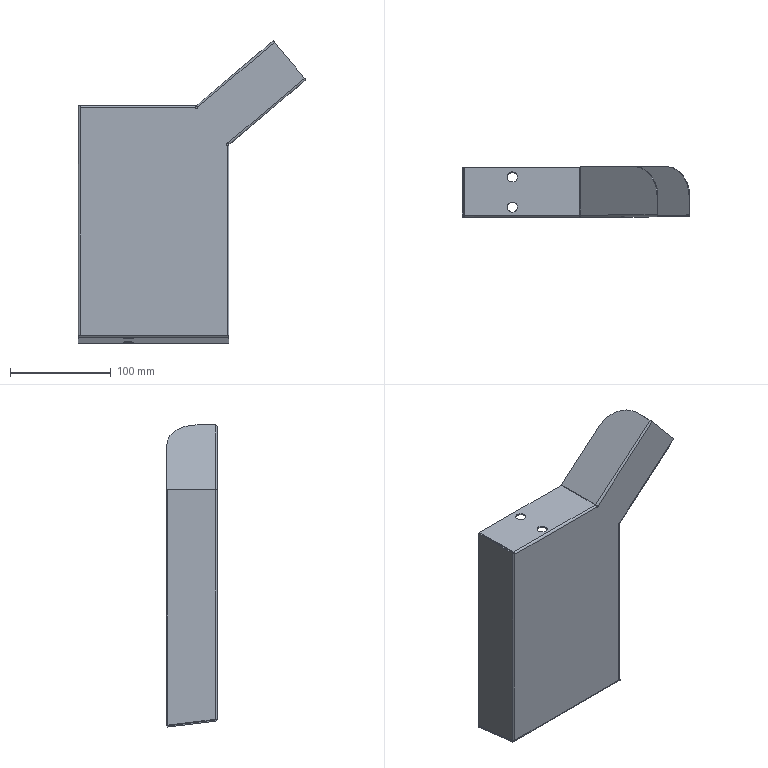Part | 1 solid | 82 faces | box 226.46 x 50 x 300.397 mm | volume 97122 mm3 | plane 58 | cylinder 22 | spline 2 | commonest cylinder face diameters 10 x8 1.473 x6 3.873 x6 60 x2